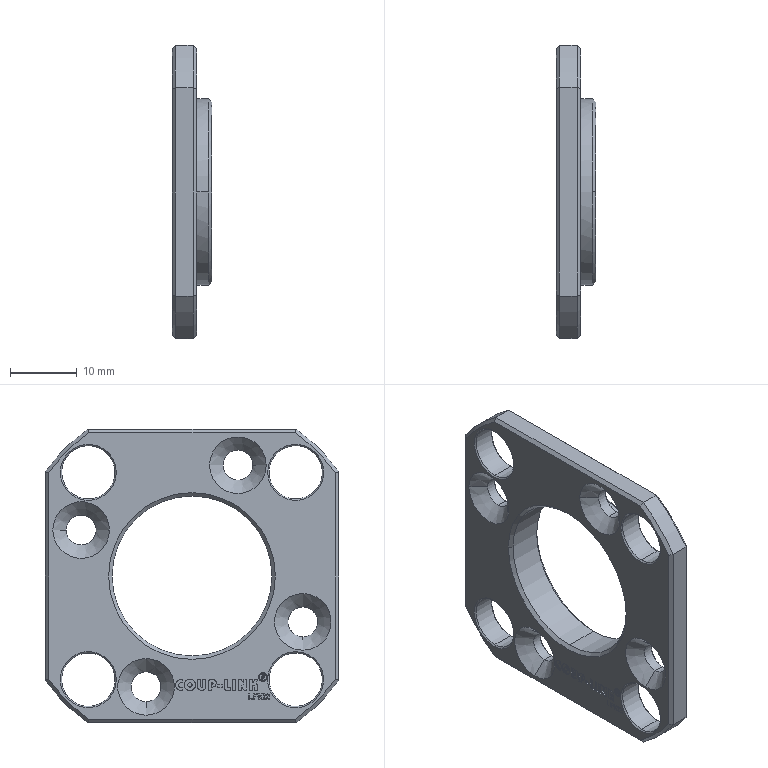Part | STEP file | LFK12-GAI-1 | 1 solid | 697 faces | box 6 x 44 x 44 mm | volume 4397 mm3 | plane 627 | cone 46 | cylinder 24 | commonest cylinder face diameters 4.5 x8 8 x8 54 x4 24 x2 28 x2